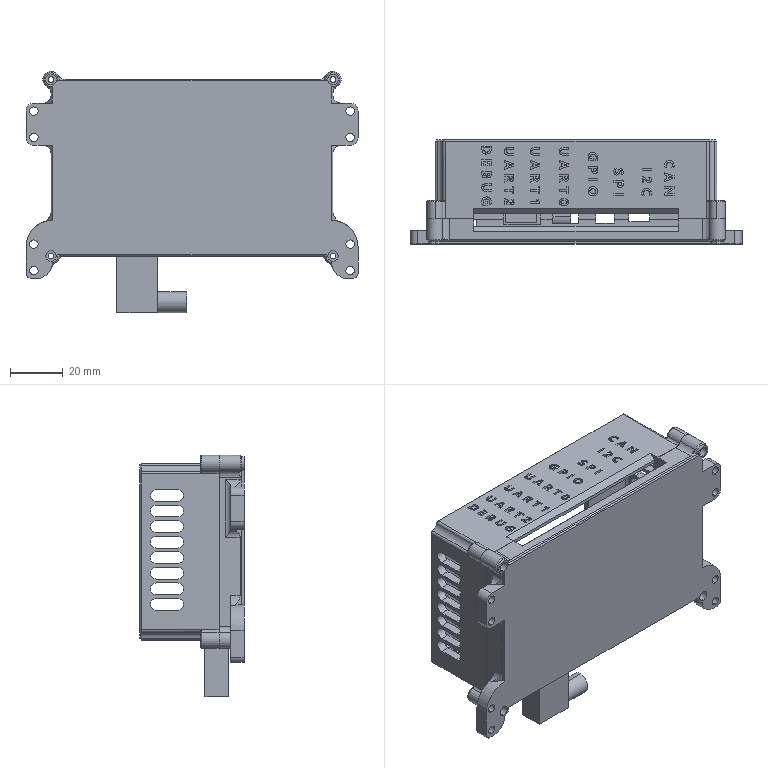Part | SolidWorks | 3 solids | 1108 faces | box 126 x 39.5 x 91.6 mm | volume 67574 mm3 | plane 613 | spline 234 | cylinder 229 | cone 20 | sphere 8 | torus 4 | commonest cylinder face diameters 2 x56 4.5 x32 5 x22 6 x22 3.2 x17 2.2 x16